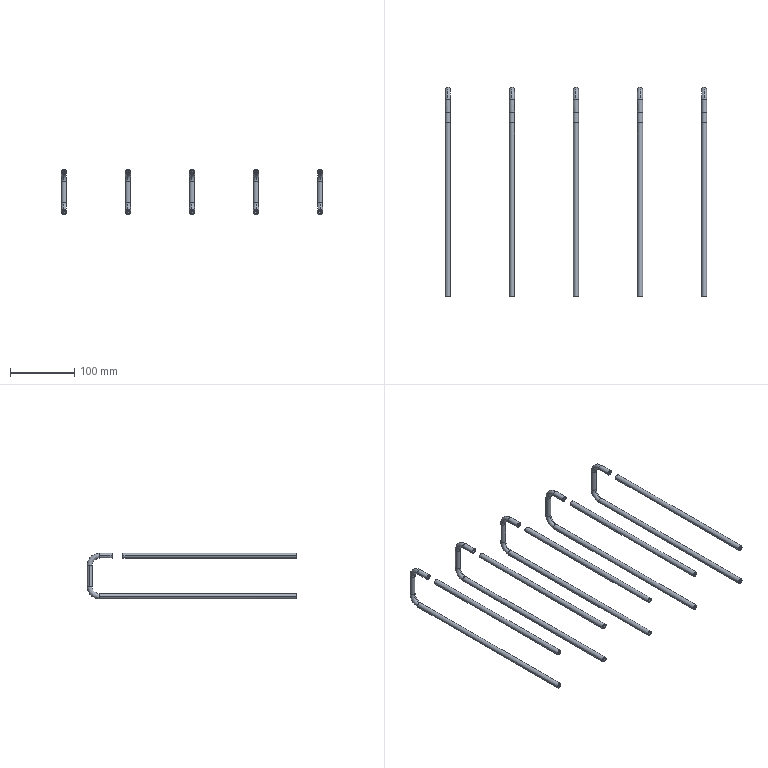Part | SolidWorks | 10 solids | 140 faces | box 408 x 327.5 x 71.18 mm | volume 128215 mm3 | cylinder 80 | torus 40 | plane 20 | commonest cylinder face diameters 4 x40 8 x40